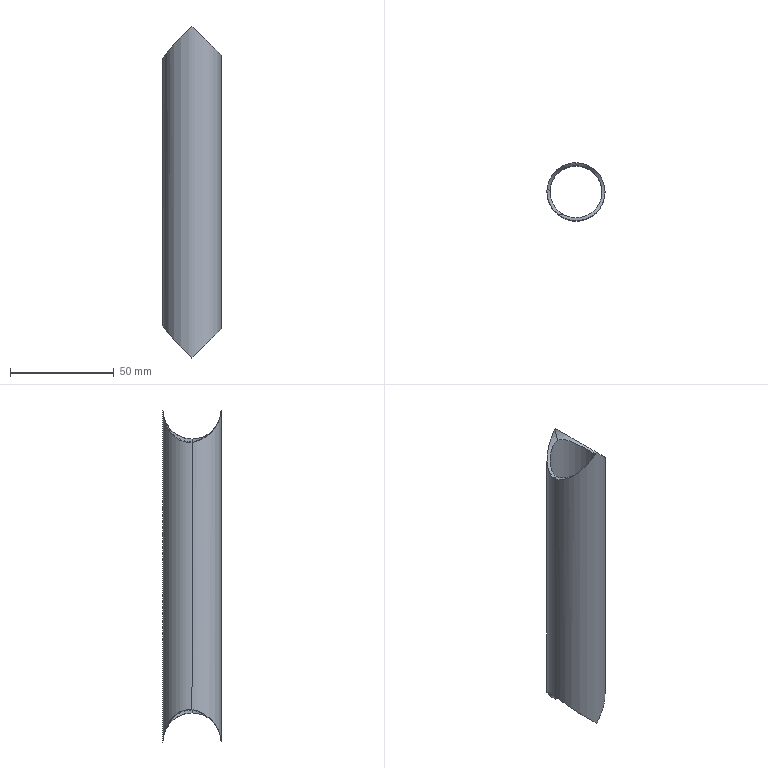Part | STEP file | PRT0001_68_16 | 1 solid | 10 faces | box 28 x 28 x 159.999 mm | volume 17361 mm3 | cylinder 6 | spline 4 | commonest cylinder face diameters 28 x4 25.014 x2